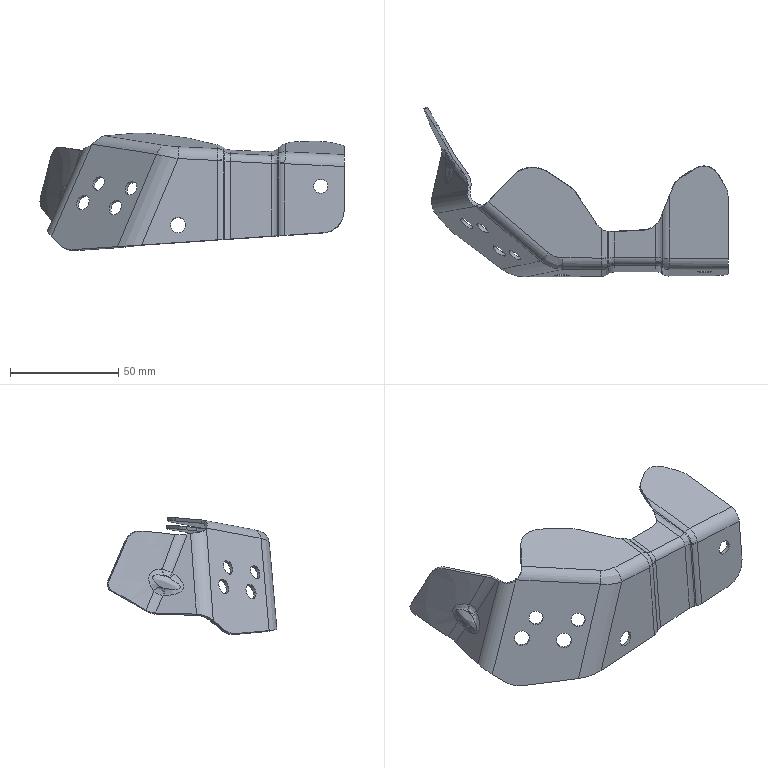Part | 1 solid | 179 faces | box 140.195 x 78.224 x 54.131 mm | volume 15752 mm3 | spline 108 | cylinder 45 | plane 26 | commonest cylinder face diameters 7 x10 10 x8 6.5 x6 13 x5 8 x3 9 x3